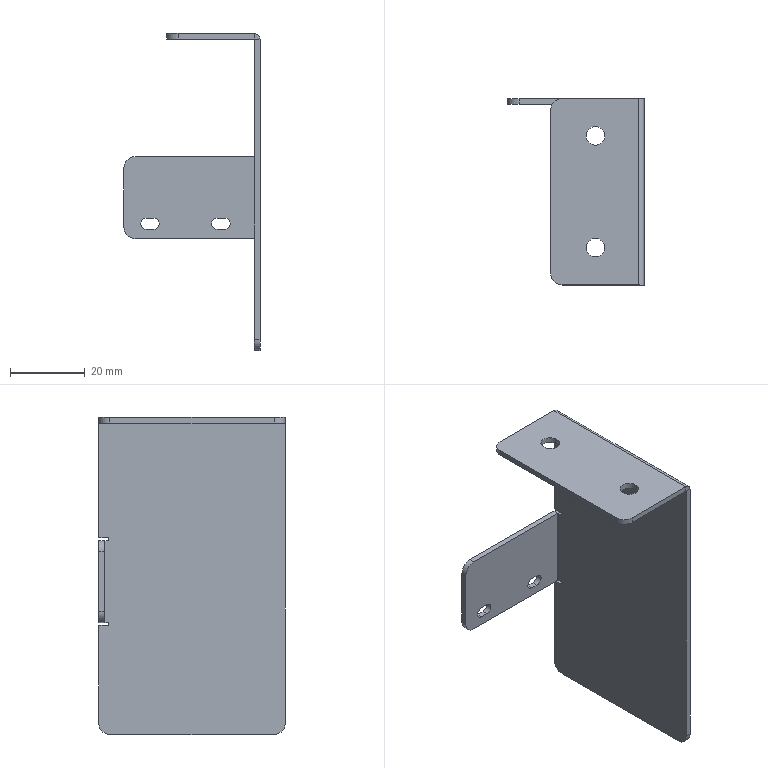Part | SolidWorks | features EdgeFlange 2, HoleWzd 2, Fillet 1, FlatPattern 1, SMBaseFlange 1, SheetMetal 1 | 1 solid | 48 faces | box 36.5 x 50 x 85 mm | volume 9132 mm3 | plane 28 | cylinder 20 | commonest cylinder face diameters 6 x6 3 x4 5 x4 0.2 x2 0.75 x2 3.2 x2
STEP:
#1=CARTESIAN_POINT('',(-15.5,15.,26.5));
#2=VERTEX_POINT('',#1);
#3=CARTESIAN_POINT('',(-10.5,15.,26.5));
#4=VERTEX_POINT('',#3);
#5=CARTESIAN_POINT('',(-13.,15.,26.5));
#6=DIRECTION('',(0.,0.,1.));
#7=DIRECTION('',(1.,0.,0.));
#8=AXIS2_PLACEMENT_3D('',#5,#6,#7);
#9=CIRCLE('',#8,2.5);
#10=EDGE_CURVE('',#2,#4,#9,.T.);
#11=ORIENTED_EDGE('',*,*,#10,.F.);
#12=CARTESIAN_POINT('',(-15.5,15.,28.));
#13=VERTEX_POINT('',#12);
#14=CARTESIAN_POINT('',(-15.5,15.,28.));
#15=DIRECTION('',(0.,0.,1.));
#16=VECTOR('',#15,1000.);
#17=LINE('',#14,#16);
#18=EDGE_CURVE('',#2,#13,#17,.T.);
#19=ORIENTED_EDGE('',*,*,#18,.T.);
#20=CARTESIAN_POINT('',(-10.5,15.,28.));
#21=VERTEX_POINT('',#20);
#22=CARTESIAN_POINT('',(-13.,15.,28.));
#23=DIRECTION('',(0.,0.,1.));
#24=DIRECTION('',(1.,0.,0.));
#25=AXIS2_PLACEMENT_3D('',#22,#23,#24);
#26=CIRCLE('',#25,2.5);
#27=EDGE_CURVE('',#13,#21,#26,.T.);
#28=ORIENTED_EDGE('',*,*,#27,.T.);
#29=CARTESIAN_POINT('',(-10.5,15.,28.));
#30=DIRECTION('',(0.,0.,1.));
#31=VECTOR('',#30,1000.);
#32=LINE('',#29,#31);
#33=EDGE_CURVE('',#4,#21,#32,.T.);
#34=ORIENTED_EDGE('',*,*,#33,.F.);
#35=EDGE_LOOP('',(#11,#19,#28,#34));
#36=FACE_OUTER_BOUND('',#35,.T.);
#37=CARTESIAN_POINT('',(-13.,15.,28.));
#38=DIRECTION('',(0.,0.,1.));
#39=DIRECTION('',(1.,0.,0.));
#40=AXIS2_PLACEMENT_3D('',#37,#38,#39);
#41=CYLINDRICAL_SURFACE('',#40,2.5);
#42=ADVANCED_FACE('',(#36),#41,.F.);
#43=CARTESIAN_POINT('',(-15.5,-15.,26.5));
#44=VERTEX_POINT('',#43);
#45=CARTESIAN_POINT('',(-10.5,-15.,26.5));
#46=VERTEX_POINT('',#45);
#47=CARTESIAN_POINT('',(-13.,-15.,26.5));
#48=DIRECTION('',(0.,0.,1.));
#49=DIRECTION('',(1.,0.,0.));
#50=AXIS2_PLACEMENT_3D('',#47,#48,#49);
#51=CIRCLE('',#50,2.5);
#52=EDGE_CURVE('',#44,#46,#51,.T.);
#53=ORIENTED_EDGE('',*,*,#52,.F.);
#54=CARTESIAN_POINT('',(-15.5,-15.,28.));
#55=VERTEX_POINT('',#54);
#56=CARTESIAN_POINT('',(-15.5,-15.,28.));
#57=DIRECTION('',(0.,0.,1.));
#58=VECTOR('',#57,1000.);
#59=LINE('',#56,#58);
#60=EDGE_CURVE('',#44,#55,#59,.T.);
#61=ORIENTED_EDGE('',*,*,#60,.T.);
#62=CARTESIAN_POINT('',(-10.5,-15.,28.));
#63=VERTEX_POINT('',#62);
#64=CARTESIAN_POINT('',(-13.,-15.,28.));
#65=DIRECTION('',(0.,0.,1.));
#66=DIRECTION('',(1.,0.,0.));
#67=AXIS2_PLACEMENT_3D('',#64,#65,#66);
#68=CIRCLE('',#67,2.5);
#69=EDGE_CURVE('',#55,#63,#68,.T.);
#70=ORIENTED_EDGE('',*,*,#69,.T.);
#71=CARTESIAN_POINT('',(-10.5,-15.,28.));
#72=DIRECTION('',(0.,0.,1.));
#73=VECTOR('',#72,1000.);
#74=LINE('',#71,#73);
#75=EDGE_CURVE('',#46,#63,#74,.T.);
#76=ORIENTED_EDGE('',*,*,#75,.F.);
#77=EDGE_LOOP('',(#53,#61,#70,#76));
#78=FACE_OUTER_BOUND('',#77,.T.);
#79=CARTESIAN_POINT('',(-13.,-15.,28.));
#80=DIRECTION('',(0.,0.,1.));
#81=DIRECTION('',(1.,0.,0.));
#82=AXIS2_PLACEMENT_3D('',#79,#80,#81);
#83=CYLINDRICAL_SURFACE('',#82,2.5);
#84=ADVANCED_FACE('',(#78),#83,.F.);
#85=CARTESIAN_POINT('',(0.,25.,-54.));
#86=VERTEX_POINT('',#85);
#87=CARTESIAN_POINT('',(0.,25.,-27.75));
#88=VERTEX_POINT('',#87);
#89=CARTESIAN_POINT('',(0.,25.,-57.));
#90=DIRECTION('',(0.,0.,1.));
#91=VECTOR('',#90,1000.);
#92=LINE('',#89,#91);
#93=EDGE_CURVE('',#86,#88,#92,.T.);
#94=ORIENTED_EDGE('',*,*,#93,.F.);
#95=CARTESIAN_POINT('',(-1.5,25.,-54.));
#96=VERTEX_POINT('',#95);
#97=CARTESIAN_POINT('',(-1.5,25.,-54.));
#98=DIRECTION('',(-1.,0.,0.));
#99=VECTOR('',#98,1000.);
#100=LINE('',#97,#99);
#101=EDGE_CURVE('',#86,#96,#100,.T.);
#102=ORIENTED_EDGE('',*,*,#101,.T.);
#103=CARTESIAN_POINT('',(-1.5,25.,-27.75));
#104=VERTEX_POINT('',#103);
#105=CARTESIAN_POINT('',(-1.5,25.,-57.));
#106=DIRECTION('',(0.,0.,1.));
#107=VECTOR('',#106,1000.);
#108=LINE('',#105,#107);
#109=EDGE_CURVE('',#96,#104,#108,.T.);
#110=ORIENTED_EDGE('',*,*,#109,.T.);
#111=CARTESIAN_POINT('',(-1.5,25.,-27.75));
#112=DIRECTION('',(1.,0.,0.));
#113=VECTOR('',#112,1000.);
#114=LINE('',#111,#113);
#115=EDGE_CURVE('',#104,#88,#114,.T.);
#116=ORIENTED_EDGE('',*,*,#115,.T.);
#117=EDGE_LOOP('',(#94,#102,#110,#116));
#118=FACE_OUTER_BOUND('',#117,.T.);
#119=CARTESIAN_POINT('',(-1.5,25.,-57.));
#120=DIRECTION('',(0.,1.,0.));
#121=DIRECTION('',(0.,0.,1.));
#122=AXIS2_PLACEMENT_3D('',#119,#120,#121);
#123=PLANE('',#122);
#124=ADVANCED_FACE('',(#118),#123,.T.);
#125=CARTESIAN_POINT('',(0.,25.,-4.25));
#126=VERTEX_POINT('',#125);
#127=CARTESIAN_POINT('',(0.,25.,26.4));
#128=VERTEX_POINT('',#127);
#129=CARTESIAN_POINT('',(0.,25.,-57.));
#130=DIRECTION('',(0.,0.,1.));
#131=VECTOR('',#130,1000.);
#132=LINE('',#129,#131);
#133=EDGE_CURVE('',#126,#128,#132,.T.);
#134=ORIENTED_EDGE('',*,*,#133,.F.);
#135=CARTESIAN_POINT('',(-1.5,25.,-4.25));
#136=VERTEX_POINT('',#135);
#137=CARTESIAN_POINT('',(-1.5,25.,-4.25));
#138=DIRECTION('',(1.,0.,0.));
#139=VECTOR('',#138,1000.);
#140=LINE('',#137,#139);
#141=EDGE_CURVE('',#136,#126,#140,.T.);
#142=ORIENTED_EDGE('',*,*,#141,.F.);
#143=CARTESIAN_POINT('',(-1.5,25.,26.4));
#144=VERTEX_POINT('',#143);
#145=CARTESIAN_POINT('',(-1.5,25.,-57.));
#146=DIRECTION('',(0.,0.,1.));
#147=VECTOR('',#146,1000.);
#148=LINE('',#145,#147);
#149=EDGE_CURVE('',#136,#144,#148,.T.);
#150=ORIENTED_EDGE('',*,*,#149,.T.);
#151=CARTESIAN_POINT('',(-1.5,25.,26.4));
#152=DIRECTION('',(1.,0.,0.));
#153=VECTOR('',#152,1000.);
#154=LINE('',#151,#153);
#155=EDGE_CURVE('',#144,#128,#154,.T.);
#156=ORIENTED_EDGE('',*,*,#155,.T.);
#157=EDGE_LOOP('',(#134,#142,#150,#156));
#158=FACE_OUTER_BOUND('',#157,.T.);
#159=CARTESIAN_POINT('',(-1.5,25.,-57.));
#160=DIRECTION('',(0.,1.,0.));
#161=DIRECTION('',(0.,0.,1.));
#162=AXIS2_PLACEMENT_3D('',#159,#160,#161);
#163=PLANE('',#162);
#164=ADVANCED_FACE('',(#158),#163,.T.);
#165=CARTESIAN_POINT('',(-1.5,-22.,-57.));
#166=VERTEX_POINT('',#165);
#167=CARTESIAN_POINT('',(-1.5,22.,-57.));
#168=VERTEX_POINT('',#167);
#169=CARTESIAN_POINT('',(-1.5,-25.,-57.));
#170=DIRECTION('',(0.,1.,0.));
#171=VECTOR('',#170,1000.);
#172=LINE('',#169,#171);
#173=EDGE_CURVE('',#166,#168,#172,.T.);
#174=ORIENTED_EDGE('',*,*,#173,.F.);
#175=CARTESIAN_POINT('',(-1.5,-25.,-54.));
#176=VERTEX_POINT('',#175);
#177=CARTESIAN_POINT('',(-1.5,-22.,-54.));
#178=DIRECTION('',(-1.,0.,0.));
#179=DIRECTION('',(0.,0.,-1.));
#180=AXIS2_PLACEMENT_3D('',#177,#178,#179);
#181=CIRCLE('',#180,3.);
#182=EDGE_CURVE('',#166,#176,#181,.T.);
#183=ORIENTED_EDGE('',*,*,#182,.T.);
#184=CARTESIAN_POINT('',(-1.5,-25.,26.4));
#185=VERTEX_POINT('',#184);
#186=CARTESIAN_POINT('',(-1.5,-25.,-57.));
#187=DIRECTION('',(0.,0.,-1.));
#188=VECTOR('',#187,1000.);
#189=LINE('',#186,#188);
#190=EDGE_CURVE('',#185,#176,#189,.T.);
#191=ORIENTED_EDGE('',*,*,#190,.F.);
#192=CARTESIAN_POINT('',(-1.5,25.,26.4));
#193=DIRECTION('',(0.,-1.,0.));
#194=VECTOR('',#193,1000.);
#195=LINE('',#192,#194);
#196=EDGE_CURVE('',#144,#185,#195,.T.);
#197=ORIENTED_EDGE('',*,*,#196,.F.);
#198=ORIENTED_EDGE('',*,*,#149,.F.);
#199=CARTESIAN_POINT('',(-1.5,22.65,-4.25));
#200=VERTEX_POINT('',#199);
#201=CARTESIAN_POINT('',(-1.5,22.65,-4.25));
#202=DIRECTION('',(0.,1.,0.));
#203=VECTOR('',#202,1000.);
#204=LINE('',#201,#203);
#205=EDGE_CURVE('',#200,#136,#204,.T.);
#206=ORIENTED_EDGE('',*,*,#205,.F.);
#207=CARTESIAN_POINT('',(-1.5,22.65,-5.));
#208=VERTEX_POINT('',#207);
#209=CARTESIAN_POINT('',(-1.5,22.65,-4.625));
#210=DIRECTION('',(-1.,0.,0.));
#211=DIRECTION('',(0.,0.,1.));
#212=AXIS2_PLACEMENT_3D('',#209,#210,#211);
#213=CIRCLE('',#212,0.375);
#214=EDGE_CURVE('',#208,#200,#213,.T.);
#215=ORIENTED_EDGE('',*,*,#214,.F.);
#216=CARTESIAN_POINT('',(-1.5,23.4,-5.));
#217=VERTEX_POINT('',#216);
#218=CARTESIAN_POINT('',(-1.5,23.4,-5.));
#219=DIRECTION('',(0.,-1.,0.));
#220=VECTOR('',#219,1000.);
#221=LINE('',#218,#220);
#222=EDGE_CURVE('',#217,#208,#221,.T.);
#223=ORIENTED_EDGE('',*,*,#222,.F.);
#224=CARTESIAN_POINT('',(-1.5,23.4,-27.));
#225=VERTEX_POINT('',#224);
#226=CARTESIAN_POINT('',(-1.5,23.4,-27.));
#227=DIRECTION('',(0.,0.,1.));
#228=VECTOR('',#227,1000.);
#229=LINE('',#226,#228);
#230=EDGE_CURVE('',#225,#217,#229,.T.);
#231=ORIENTED_EDGE('',*,*,#230,.F.);
#232=CARTESIAN_POINT('',(-1.5,22.65,-27.));
#233=VERTEX_POINT('',#232);
#234=CARTESIAN_POINT('',(-1.5,22.65,-27.));
#235=DIRECTION('',(0.,1.,0.));
#236=VECTOR('',#235,1000.);
#237=LINE('',#234,#236);
#238=EDGE_CURVE('',#233,#225,#237,.T.);
#239=ORIENTED_EDGE('',*,*,#238,.F.);
#240=CARTESIAN_POINT('',(-1.5,22.65,-27.75));
#241=VERTEX_POINT('',#240);
#242=CARTESIAN_POINT('',(-1.5,22.65,-27.375));
#243=DIRECTION('',(-1.,0.,0.));
#244=DIRECTION('',(0.,0.,1.));
#245=AXIS2_PLACEMENT_3D('',#242,#243,#244);
#246=CIRCLE('',#245,0.375);
#247=EDGE_CURVE('',#241,#233,#246,.T.);
#248=ORIENTED_EDGE('',*,*,#247,.F.);
#249=CARTESIAN_POINT('',(-1.5,25.,-27.75));
#250=DIRECTION('',(0.,-1.,0.));
#251=VECTOR('',#250,1000.);
#252=LINE('',#249,#251);
#253=EDGE_CURVE('',#104,#241,#252,.T.);
#254=ORIENTED_EDGE('',*,*,#253,.F.);
#255=ORIENTED_EDGE('',*,*,#109,.F.);
#256=CARTESIAN_POINT('',(-1.5,22.,-54.));
#257=DIRECTION('',(-1.,0.,0.));
#258=DIRECTION('',(0.,0.,-1.));
#259=AXIS2_PLACEMENT_3D('',#256,#257,#258);
#260=CIRCLE('',#259,3.);
#261=EDGE_CURVE('',#96,#168,#260,.T.);
#262=ORIENTED_EDGE('',*,*,#261,.T.);
#263=EDGE_LOOP('',(#174,#183,#191,#197,#198,#206,#215,#223,#231,#239,#248,#254,#255,#262));
#264=FACE_OUTER_BOUND('',#263,.T.);
#265=CARTESIAN_POINT('',(-1.5,0.,0.));
#266=DIRECTION('',(1.,0.,0.));
#267=DIRECTION('',(0.,0.,-1.));
#268=AXIS2_PLACEMENT_3D('',#265,#266,#267);
#269=PLANE('',#268);
#270=ADVANCED_FACE('',(#264),#269,.F.);
#271=CARTESIAN_POINT('',(0.,-25.,26.4));
#272=VERTEX_POINT('',#271);
#273=CARTESIAN_POINT('',(0.,-25.,-54.));
#274=VERTEX_POINT('',#273);
#275=CARTESIAN_POINT('',(0.,-25.,-57.));
#276=DIRECTION('',(0.,0.,-1.));
#277=VECTOR('',#276,1000.);
#278=LINE('',#275,#277);
#279=EDGE_CURVE('',#272,#274,#278,.T.);
#280=ORIENTED_EDGE('',*,*,#279,.T.);
#281=CARTESIAN_POINT('',(0.,-22.,-57.));
#282=VERTEX_POINT('',#281);
#283=CARTESIAN_POINT('',(0.,-22.,-54.));
#284=DIRECTION('',(1.,0.,0.));
#285=DIRECTION('',(0.,0.,-1.));
#286=AXIS2_PLACEMENT_3D('',#283,#284,#285);
#287=CIRCLE('',#286,3.);
#288=EDGE_CURVE('',#274,#282,#287,.T.);
#289=ORIENTED_EDGE('',*,*,#288,.T.);
#290=CARTESIAN_POINT('',(0.,22.,-57.));
#291=VERTEX_POINT('',#290);
#292=CARTESIAN_POINT('',(0.,-25.,-57.));
#293=DIRECTION('',(0.,1.,0.));
#294=VECTOR('',#293,1000.);
#295=LINE('',#292,#294);
#296=EDGE_CURVE('',#282,#291,#295,.T.);
#297=ORIENTED_EDGE('',*,*,#296,.T.);
#298=CARTESIAN_POINT('',(0.,22.,-54.));
#299=DIRECTION('',(1.,0.,0.));
#300=DIRECTION('',(0.,0.,-1.));
#301=AXIS2_PLACEMENT_3D('',#298,#299,#300);
#302=CIRCLE('',#301,3.);
#303=EDGE_CURVE('',#291,#86,#302,.T.);
#304=ORIENTED_EDGE('',*,*,#303,.T.);
#305=ORIENTED_EDGE('',*,*,#93,.T.);
#306=CARTESIAN_POINT('',(0.,22.65,-27.75));
#307=VERTEX_POINT('',#306);
#308=CARTESIAN_POINT('',(0.,0.,-27.75));
#309=DIRECTION('',(0.,-1.,0.));
#310=VECTOR('',#309,1000.);
#311=LINE('',#308,#310);
#312=EDGE_CURVE('',#88,#307,#311,.T.);
#313=ORIENTED_EDGE('',*,*,#312,.T.);
#314=CARTESIAN_POINT('',(0.,22.65,-27.));
#315=VERTEX_POINT('',#314);
#316=CARTESIAN_POINT('',(0.,22.65,-27.375));
#317=DIRECTION('',(-1.,0.,0.));
#318=DIRECTION('',(0.,0.,-1.));
#319=AXIS2_PLACEMENT_3D('',#316,#317,#318);
#320=CIRCLE('',#319,0.375);
#321=EDGE_CURVE('',#307,#315,#320,.T.);
#322=ORIENTED_EDGE('',*,*,#321,.T.);
#323=CARTESIAN_POINT('',(0.,23.4,-27.));
#324=VERTEX_POINT('',#323);
#325=CARTESIAN_POINT('',(0.,0.,-27.));
#326=DIRECTION('',(0.,1.,0.));
#327=VECTOR('',#326,1000.);
#328=LINE('',#325,#327);
#329=EDGE_CURVE('',#315,#324,#328,.T.);
#330=ORIENTED_EDGE('',*,*,#329,.T.);
#331=CARTESIAN_POINT('',(0.,23.4,-5.));
#332=VERTEX_POINT('',#331);
#333=CARTESIAN_POINT('',(0.,23.4,-27.));
#334=DIRECTION('',(0.,0.,1.));
#335=VECTOR('',#334,1000.);
#336=LINE('',#333,#335);
#337=EDGE_CURVE('',#324,#332,#336,.T.);
#338=ORIENTED_EDGE('',*,*,#337,.T.);
#339=CARTESIAN_POINT('',(0.,22.65,-5.));
#340=VERTEX_POINT('',#339);
#341=CARTESIAN_POINT('',(0.,0.,-5.));
#342=DIRECTION('',(0.,-1.,0.));
#343=VECTOR('',#342,1000.);
#344=LINE('',#341,#343);
#345=EDGE_CURVE('',#332,#340,#344,.T.);
#346=ORIENTED_EDGE('',*,*,#345,.T.);
#347=CARTESIAN_POINT('',(0.,22.65,-4.25));
#348=VERTEX_POINT('',#347);
#349=CARTESIAN_POINT('',(0.,22.65,-4.625));
#350=DIRECTION('',(-1.,0.,0.));
#351=DIRECTION('',(0.,0.,-1.));
#352=AXIS2_PLACEMENT_3D('',#349,#350,#351);
#353=CIRCLE('',#352,0.375);
#354=EDGE_CURVE('',#340,#348,#353,.T.);
#355=ORIENTED_EDGE('',*,*,#354,.T.);
#356=CARTESIAN_POINT('',(0.,0.,-4.25));
#357=DIRECTION('',(0.,1.,0.));
#358=VECTOR('',#357,1000.);
#359=LINE('',#356,#358);
#360=EDGE_CURVE('',#348,#126,#359,.T.);
#361=ORIENTED_EDGE('',*,*,#360,.T.);
#362=ORIENTED_EDGE('',*,*,#133,.T.);
#363=CARTESIAN_POINT('',(0.,25.,26.4));
#364=DIRECTION('',(0.,-1.,0.));
#365=VECTOR('',#364,1000.);
#366=LINE('',#363,#365);
#367=EDGE_CURVE('',#128,#272,#366,.T.);
#368=ORIENTED_EDGE('',*,*,#367,.T.);
#369=EDGE_LOOP('',(#280,#289,#297,#304,#305,#313,#322,#330,#338,#346,#355,#361,#362,#368));
#370=FACE_OUTER_BOUND('',#369,.T.);
#371=CARTESIAN_POINT('',(0.,0.,0.));
#372=DIRECTION('',(1.,0.,0.));
#373=DIRECTION('',(0.,0.,-1.));
#374=AXIS2_PLACEMENT_3D('',#371,#372,#373);
#375=PLANE('',#374);
#376=ADVANCED_FACE('',(#370),#375,.T.);
#377=ORIENTED_EDGE('',*,*,#296,.F.);
#378=CARTESIAN_POINT('',(-1.5,-22.,-57.));
#379=DIRECTION('',(-1.,0.,0.));
#380=VECTOR('',#379,1000.);
#381=LINE('',#378,#380);
#382=EDGE_CURVE('',#282,#166,#381,.T.);
#383=ORIENTED_EDGE('',*,*,#382,.T.);
#384=ORIENTED_EDGE('',*,*,#173,.T.);
#385=CARTESIAN_POINT('',(-1.5,22.,-57.));
#386=DIRECTION('',(1.,0.,0.));
#387=VECTOR('',#386,1000.);
#388=LINE('',#385,#387);
#389=EDGE_CURVE('',#168,#291,#388,.T.);
#390=ORIENTED_EDGE('',*,*,#389,.T.);
#391=EDGE_LOOP('',(#377,#383,#384,#390));
#392=FACE_OUTER_BOUND('',#391,.T.);
#393=CARTESIAN_POINT('',(-1.5,-25.,-57.));
#394=DIRECTION('',(0.,0.,-1.));
#395=DIRECTION('',(-1.,0.,0.));
#396=AXIS2_PLACEMENT_3D('',#393,#394,#395);
#397=PLANE('',#396);
#398=ADVANCED_FACE('',(#392),#397,.T.);
#399=ORIENTED_EDGE('',*,*,#190,.T.);
#400=CARTESIAN_POINT('',(-1.5,-25.,-54.));
#401=DIRECTION('',(1.,0.,0.));
#402=VECTOR('',#401,1000.);
#403=LINE('',#400,#402);
#404=EDGE_CURVE('',#176,#274,#403,.T.);
#405=ORIENTED_EDGE('',*,*,#404,.T.);
#406=ORIENTED_EDGE('',*,*,#279,.F.);
#407=CARTESIAN_POINT('',(-1.5,-25.,26.4));
#408=DIRECTION('',(1.,0.,0.));
#409=VECTOR('',#408,1000.);
#410=LINE('',#407,#409);
#411=EDGE_CURVE('',#185,#272,#410,.T.);
#412=ORIENTED_EDGE('',*,*,#411,.F.);
#413=EDGE_LOOP('',(#399,#405,#406,#412));
#414=FACE_OUTER_BOUND('',#413,.T.);
#415=CARTESIAN_POINT('',(-1.5,-25.,-57.));
#416=DIRECTION('',(0.,-1.,0.));
#417=DIRECTION('',(0.,0.,-1.));
#418=AXIS2_PLACEMENT_3D('',#415,#416,#417);
#419=PLANE('',#418);
#420=ADVANCED_FACE('',(#414),#419,.T.);
#421=CARTESIAN_POINT('',(-1.6,-25.,26.5));
#422=VERTEX_POINT('',#421);
#423=CARTESIAN_POINT('',(-1.6,-25.,28.));
#424=VERTEX_POINT('',#423);
#425=CARTESIAN_POINT('',(-1.6,-25.,28.));
#426=DIRECTION('',(0.,0.,1.));
#427=VECTOR('',#426,1000.);
#428=LINE('',#425,#427);
#429=EDGE_CURVE('',#422,#424,#428,.T.);
#430=ORIENTED_EDGE('',*,*,#429,.F.);
#431=CARTESIAN_POINT('',(-1.6,-25.,26.4));
#432=DIRECTION('',(0.,-1.,0.));
#433=DIRECTION('',(0.,0.,1.));
#434=AXIS2_PLACEMENT_3D('',#431,#432,#433);
#435=CIRCLE('',#434,0.1);
#436=EDGE_CURVE('',#185,#422,#435,.T.);
#437=ORIENTED_EDGE('',*,*,#436,.F.);
#438=ORIENTED_EDGE('',*,*,#411,.T.);
#439=CARTESIAN_POINT('',(-1.6,-25.,26.4));
#440=DIRECTION('',(0.,-1.,0.));
#441=DIRECTION('',(0.,0.,1.));
#442=AXIS2_PLACEMENT_3D('',#439,#440,#441);
#443=CIRCLE('',#442,1.6);
#444=EDGE_CURVE('',#272,#424,#443,.T.);
#445=ORIENTED_EDGE('',*,*,#444,.T.);
#446=EDGE_LOOP('',(#430,#437,#438,#445));
#447=FACE_OUTER_BOUND('',#446,.T.);
#448=CARTESIAN_POINT('',(-1.6,-25.,26.4));
#449=DIRECTION('',(0.,-1.,0.));
#450=DIRECTION('',(0.,0.,-1.));
#451=AXIS2_PLACEMENT_3D('',#448,#449,#450);
#452=PLANE('',#451);
#453=ADVANCED_FACE('',(#447),#452,.T.);
#454=CARTESIAN_POINT('',(-1.6,25.,26.5));
#455=VERTEX_POINT('',#454);
#456=CARTESIAN_POINT('',(-1.6,25.,26.4));
#457=DIRECTION('',(0.,1.,0.));
#458=DIRECTION('',(0.,0.,1.));
#459=AXIS2_PLACEMENT_3D('',#456,#457,#458);
#460=CIRCLE('',#459,0.1);
#461=EDGE_CURVE('',#455,#144,#460,.T.);
#462=ORIENTED_EDGE('',*,*,#461,.F.);
#463=CARTESIAN_POINT('',(-1.6,25.,28.));
#464=VERTEX_POINT('',#463);
#465=CARTESIAN_POINT('',(-1.6,25.,26.5));
#466=DIRECTION('',(0.,0.,1.));
#467=VECTOR('',#466,1000.);
#468=LINE('',#465,#467);
#469=EDGE_CURVE('',#455,#464,#468,.T.);
#470=ORIENTED_EDGE('',*,*,#469,.T.);
#471=CARTESIAN_POINT('',(-1.6,25.,26.4));
#472=DIRECTION('',(0.,1.,0.));
#473=DIRECTION('',(0.,0.,1.));
#474=AXIS2_PLACEMENT_3D('',#471,#472,#473);
#475=CIRCLE('',#474,1.6);
#476=EDGE_CURVE('',#464,#128,#475,.T.);
#477=ORIENTED_EDGE('',*,*,#476,.T.);
#478=ORIENTED_EDGE('',*,*,#155,.F.);
#479=EDGE_LOOP('',(#462,#470,#477,#478));
#480=FACE_OUTER_BOUND('',#479,.T.);
#481=CARTESIAN_POINT('',(-1.6,25.,26.4));
#482=DIRECTION('',(0.,-1.,0.));
#483=DIRECTION('',(0.,0.,-1.));
#484=AXIS2_PLACEMENT_3D('',#481,#482,#483);
#485=PLANE('',#484);
#486=ADVANCED_FACE('',(#480),#485,.F.);
#487=ORIENTED_EDGE('',*,*,#367,.F.);
#488=ORIENTED_EDGE('',*,*,#476,.F.);
#489=CARTESIAN_POINT('',(-1.6,0.,28.));
#490=DIRECTION('',(0.,1.,0.));
#491=VECTOR('',#490,1000.);
#492=LINE('',#489,#491);
#493=EDGE_CURVE('',#424,#464,#492,.T.);
#494=ORIENTED_EDGE('',*,*,#493,.F.);
#495=ORIENTED_EDGE('',*,*,#444,.F.);
#496=EDGE_LOOP('',(#487,#488,#494,#495));
#497=FACE_OUTER_BOUND('',#496,.T.);
#498=CARTESIAN_POINT('',(-1.6,25.,26.4));
#499=DIRECTION('',(0.,1.,0.));
#500=DIRECTION('',(0.,0.,1.));
#501=AXIS2_PLACEMENT_3D('',#498,#499,#500);
#502=CYLINDRICAL_SURFACE('',#501,1.6);
#503=ADVANCED_FACE('',(#497),#502,.T.);
#504=ORIENTED_EDGE('',*,*,#196,.T.);
#505=ORIENTED_EDGE('',*,*,#436,.T.);
#506=CARTESIAN_POINT('',(-1.6,-25.,26.5));
#507=DIRECTION('',(0.,1.,0.));
#508=VECTOR('',#507,1000.);
#509=LINE('',#506,#508);
#510=EDGE_CURVE('',#422,#455,#509,.T.);
#511=ORIENTED_EDGE('',*,*,#510,.T.);
#512=ORIENTED_EDGE('',*,*,#461,.T.);
#513=EDGE_LOOP('',(#504,#505,#511,#512));
#514=FACE_OUTER_BOUND('',#513,.T.);
#515=CARTESIAN_POINT('',(-1.6,25.,26.4));
#516=DIRECTION('',(0.,1.,0.));
#517=DIRECTION('',(0.,0.,1.));
#518=AXIS2_PLACEMENT_3D('',#515,#516,#517);
#519=CYLINDRICAL_SURFACE('',#518,0.1);
#520=ADVANCED_FACE('',(#514),#519,.F.);
#521=CARTESIAN_POINT('',(-22.,25.,26.5));
#522=VERTEX_POINT('',#521);
#523=CARTESIAN_POINT('',(0.,25.,26.5));
#524=DIRECTION('',(1.,0.,0.));
#525=VECTOR('',#524,1000.);
#526=LINE('',#523,#525);
#527=EDGE_CURVE('',#522,#455,#526,.T.);
#528=ORIENTED_EDGE('',*,*,#527,.F.);
#529=CARTESIAN_POINT('',(-22.,25.,28.));
#530=VERTEX_POINT('',#529);
#531=CARTESIAN_POINT('',(-22.,25.,28.));
#532=DIRECTION('',(0.,0.,1.));
#533=VECTOR('',#532,1000.);
#534=LINE('',#531,#533);
#535=EDGE_CURVE('',#522,#530,#534,.T.);
#536=ORIENTED_EDGE('',*,*,#535,.T.);
#537=CARTESIAN_POINT('',(-1.5,25.,28.));
#538=DIRECTION('',(1.,0.,0.));
#539=VECTOR('',#538,1000.);
#540=LINE('',#537,#539);
#541=EDGE_CURVE('',#530,#464,#540,.T.);
#542=ORIENTED_EDGE('',*,*,#541,.T.);
#543=ORIENTED_EDGE('',*,*,#469,.F.);
#544=EDGE_LOOP('',(#528,#536,#542,#543));
#545=FACE_OUTER_BOUND('',#544,.T.);
#546=CARTESIAN_POINT('',(-1.5,25.,28.));
#547=DIRECTION('',(0.,1.,0.));
#548=DIRECTION('',(-1.,0.,0.));
#549=AXIS2_PLACEMENT_3D('',#546,#547,#548);
#550=PLANE('',#549);
#551=ADVANCED_FACE('',(#545),#550,.T.);
#552=CARTESIAN_POINT('',(-22.,-25.,28.));
#553=VERTEX_POINT('',#552);
#554=CARTESIAN_POINT('',(-25.,-25.,28.));
#555=DIRECTION('',(-1.,0.,0.));
#556=VECTOR('',#555,1000.);
#557=LINE('',#554,#556);
#558=EDGE_CURVE('',#424,#553,#557,.T.);
#559=ORIENTED_EDGE('',*,*,#558,.T.);
#560=CARTESIAN_POINT('',(-22.,-25.,26.5));
#561=VERTEX_POINT('',#560);
#562=CARTESIAN_POINT('',(-22.,-25.,28.));
#563=DIRECTION('',(0.,0.,-1.));
#564=VECTOR('',#563,1000.);
#565=LINE('',#562,#564);
#566=EDGE_CURVE('',#553,#561,#565,.T.);
#567=ORIENTED_EDGE('',*,*,#566,.T.);
#568=CARTESIAN_POINT('',(0.,-25.,26.5));
#569=DIRECTION('',(-1.,0.,0.));
#570=VECTOR('',#569,1000.);
#571=LINE('',#568,#570);
#572=EDGE_CURVE('',#422,#561,#571,.T.);
#573=ORIENTED_EDGE('',*,*,#572,.F.);
#574=ORIENTED_EDGE('',*,*,#429,.T.);
#575=EDGE_LOOP('',(#559,#567,#573,#574));
#576=FACE_OUTER_BOUND('',#575,.T.);
#577=CARTESIAN_POINT('',(-25.,-25.,28.));
#578=DIRECTION('',(0.,-1.,0.));
#579=DIRECTION('',(1.,0.,0.));
#580=AXIS2_PLACEMENT_3D('',#577,#578,#579);
#581=PLANE('',#580);
#582=ADVANCED_FACE('',(#576),#581,.T.);
#583=CARTESIAN_POINT('',(-13.,15.,28.));
#584=DIRECTION('',(0.,0.,1.));
#585=DIRECTION('',(1.,0.,0.));
#586=AXIS2_PLACEMENT_3D('',#583,#584,#585);
#587=CIRCLE('',#586,2.5);
#588=EDGE_CURVE('',#21,#13,#587,.T.);
#589=ORIENTED_EDGE('',*,*,#588,.F.);
#590=ORIENTED_EDGE('',*,*,#27,.F.);
#591=EDGE_LOOP('',(#589,#590));
#592=FACE_BOUND('',#591,.T.);
#593=CARTESIAN_POINT('',(-13.,-15.,28.));
#594=DIRECTION('',(0.,0.,1.));
#595=DIRECTION('',(1.,0.,0.));
#596=AXIS2_PLACEMENT_3D('',#593,#594,#595);
#597=CIRCLE('',#596,2.5);
#598=EDGE_CURVE('',#63,#55,#597,.T.);
#599=ORIENTED_EDGE('',*,*,#598,.F.);
#600=ORIENTED_EDGE('',*,*,#69,.F.);
#601=EDGE_LOOP('',(#599,#600));
#602=FACE_BOUND('',#601,.T.);
#603=CARTESIAN_POINT('',(-25.,-22.,28.));
#604=VERTEX_POINT('',#603);
#605=CARTESIAN_POINT('',(-25.,22.,28.));
#606=VERTEX_POINT('',#605);
#607=CARTESIAN_POINT('',(-25.,25.,28.));
#608=DIRECTION('',(0.,1.,0.));
#609=VECTOR('',#608,1000.);
#610=LINE('',#607,#609);
#611=EDGE_CURVE('',#604,#606,#610,.T.);
#612=ORIENTED_EDGE('',*,*,#611,.F.);
#613=CARTESIAN_POINT('',(-22.,-22.,28.));
#614=DIRECTION('',(0.,0.,1.));
#615=DIRECTION('',(1.,0.,0.));
#616=AXIS2_PLACEMENT_3D('',#613,#614,#615);
#617=CIRCLE('',#616,3.);
#618=EDGE_CURVE('',#604,#553,#617,.T.);
#619=ORIENTED_EDGE('',*,*,#618,.T.);
#620=ORIENTED_EDGE('',*,*,#558,.F.);
#621=ORIENTED_EDGE('',*,*,#493,.T.);
#622=ORIENTED_EDGE('',*,*,#541,.F.);
#623=CARTESIAN_POINT('',(-22.,22.,28.));
#624=DIRECTION('',(0.,0.,1.));
#625=DIRECTION('',(1.,0.,0.));
#626=AXIS2_PLACEMENT_3D('',#623,#624,#625);
#627=CIRCLE('',#626,3.);
#628=EDGE_CURVE('',#530,#606,#627,.T.);
#629=ORIENTED_EDGE('',*,*,#628,.T.);
#630=EDGE_LOOP('',(#612,#619,#620,#621,#622,#629));
#631=FACE_OUTER_BOUND('',#630,.T.);
#632=CARTESIAN_POINT('',(0.,0.,28.));
#633=DIRECTION('',(0.,0.,1.));
#634=DIRECTION('',(1.,0.,0.));
#635=AXIS2_PLACEMENT_3D('',#632,#633,#634);
#636=PLANE('',#635);
#637=ADVANCED_FACE('',(#592,#602,#631),#636,.T.);
#638=CARTESIAN_POINT('',(-13.,15.,26.5));
#639=DIRECTION('',(0.,0.,1.));
#640=DIRECTION('',(1.,0.,0.));
#641=AXIS2_PLACEMENT_3D('',#638,#639,#640);
#642=CIRCLE('',#641,2.5);
#643=EDGE_CURVE('',#4,#2,#642,.T.);
#644=ORIENTED_EDGE('',*,*,#643,.T.);
#645=ORIENTED_EDGE('',*,*,#10,.T.);
#646=EDGE_LOOP('',(#644,#645));
#647=FACE_BOUND('',#646,.T.);
#648=CARTESIAN_POINT('',(-13.,-15.,26.5));
#649=DIRECTION('',(0.,0.,1.));
#650=DIRECTION('',(1.,0.,0.));
#651=AXIS2_PLACEMENT_3D('',#648,#649,#650);
#652=CIRCLE('',#651,2.5);
#653=EDGE_CURVE('',#46,#44,#652,.T.);
#654=ORIENTED_EDGE('',*,*,#653,.T.);
#655=ORIENTED_EDGE('',*,*,#52,.T.);
#656=EDGE_LOOP('',(#654,#655));
#657=FACE_BOUND('',#656,.T.);
#658=ORIENTED_EDGE('',*,*,#572,.T.);
#659=CARTESIAN_POINT('',(-25.,-22.,26.5));
#660=VERTEX_POINT('',#659);
#661=CARTESIAN_POINT('',(-22.,-22.,26.5));
#662=DIRECTION('',(0.,0.,-1.));
#663=DIRECTION('',(1.,0.,0.));
#664=AXIS2_PLACEMENT_3D('',#661,#662,#663);
#665=CIRCLE('',#664,3.);
#666=EDGE_CURVE('',#561,#660,#665,.T.);
#667=ORIENTED_EDGE('',*,*,#666,.T.);
#668=CARTESIAN_POINT('',(-25.,22.,26.5));
#669=VERTEX_POINT('',#668);
#670=CARTESIAN_POINT('',(-25.,0.,26.5));
#671=DIRECTION('',(0.,1.,0.));
#672=VECTOR('',#671,1000.);
#673=LINE('',#670,#672);
#674=EDGE_CURVE('',#660,#669,#673,.T.);
#675=ORIENTED_EDGE('',*,*,#674,.T.);
#676=CARTESIAN_POINT('',(-22.,22.,26.5));
#677=DIRECTION('',(0.,0.,-1.));
#678=DIRECTION('',(1.,0.,0.));
#679=AXIS2_PLACEMENT_3D('',#676,#677,#678);
#680=CIRCLE('',#679,3.);
#681=EDGE_CURVE('',#669,#522,#680,.T.);
#682=ORIENTED_EDGE('',*,*,#681,.T.);
#683=ORIENTED_EDGE('',*,*,#527,.T.);
#684=ORIENTED_EDGE('',*,*,#510,.F.);
#685=EDGE_LOOP('',(#658,#667,#675,#682,#683,#684));
#686=FACE_OUTER_BOUND('',#685,.T.);
#687=CARTESIAN_POINT('',(0.,0.,26.5));
#688=DIRECTION('',(0.,0.,1.));
#689=DIRECTION('',(1.,0.,0.));
#690=AXIS2_PLACEMENT_3D('',#687,#688,#689);
#691=PLANE('',#690);
#692=ADVANCED_FACE('',(#647,#657,#686),#691,.F.);
#693=ORIENTED_EDGE('',*,*,#674,.F.);
#694=CARTESIAN_POINT('',(-25.,-22.,28.));
#695=DIRECTION('',(0.,0.,1.));
#696=VECTOR('',#695,1000.);
#697=LINE('',#694,#696);
#698=EDGE_CURVE('',#660,#604,#697,.T.);
#699=ORIENTED_EDGE('',*,*,#698,.T.);
#700=ORIENTED_EDGE('',*,*,#611,.T.);
#701=CARTESIAN_POINT('',(-25.,22.,28.));
#702=DIRECTION('',(0.,0.,-1.));
#703=VECTOR('',#702,1000.);
#704=LINE('',#701,#703);
#705=EDGE_CURVE('',#606,#669,#704,.T.);
#706=ORIENTED_EDGE('',*,*,#705,.T.);
#707=EDGE_LOOP('',(#693,#699,#700,#706));
#708=FACE_OUTER_BOUND('',#707,.T.);
#709=CARTESIAN_POINT('',(-25.,25.,28.));
#710=DIRECTION('',(-1.,0.,0.));
#711=DIRECTION('',(0.,0.,1.));
#712=AXIS2_PLACEMENT_3D('',#709,#710,#711);
#713=PLANE('',#712);
#714=ADVANCED_FACE('',(#708),#713,.T.);
#715=ORIENTED_EDGE('',*,*,#312,.F.);
#716=ORIENTED_EDGE('',*,*,#115,.F.);
#717=ORIENTED_EDGE('',*,*,#253,.T.);
#718=CARTESIAN_POINT('',(-1.5,22.65,-27.75));
#719=DIRECTION('',(1.,0.,0.));
#720=VECTOR('',#719,1000.);
#721=LINE('',#718,#720);
#722=EDGE_CURVE('',#241,#307,#721,.T.);
#723=ORIENTED_EDGE('',*,*,#722,.T.);
#724=EDGE_LOOP('',(#715,#716,#717,#723));
#725=FACE_OUTER_BOUND('',#724,.T.);
#726=CARTESIAN_POINT('',(-1.5,25.,-27.75));
#727=DIRECTION('',(0.,0.,1.));
#728=DIRECTION('',(1.,0.,0.));
#729=AXIS2_PLACEMENT_3D('',#726,#727,#728);
#730=PLANE('',#729);
#731=ADVANCED_FACE('',(#725),#730,.T.);
#732=ORIENTED_EDGE('',*,*,#321,.F.);
#733=ORIENTED_EDGE('',*,*,#722,.F.);
#734=ORIENTED_EDGE('',*,*,#247,.T.);
#735=CARTESIAN_POINT('',(-1.5,22.65,-27.));
#736=DIRECTION('',(1.,0.,0.));
#737=VECTOR('',#736,1000.);
#738=LINE('',#735,#737);
#739=EDGE_CURVE('',#233,#315,#738,.T.);
#740=ORIENTED_EDGE('',*,*,#739,.T.);
#741=EDGE_LOOP('',(#732,#733,#734,#740));
#742=FACE_OUTER_BOUND('',#741,.T.);
#743=CARTESIAN_POINT('',(-1.5,22.65,-27.375));
#744=DIRECTION('',(1.,0.,0.));
#745=DIRECTION('',(0.,0.,-1.));
#746=AXIS2_PLACEMENT_3D('',#743,#744,#745);
#747=CYLINDRICAL_SURFACE('',#746,0.375);
#748=ADVANCED_FACE('',(#742),#747,.F.);
#749=ORIENTED_EDGE('',*,*,#329,.F.);
#750=ORIENTED_EDGE('',*,*,#739,.F.);
#751=ORIENTED_EDGE('',*,*,#238,.T.);
#752=CARTESIAN_POINT('',(-1.5,23.4,-27.));
#753=DIRECTION('',(1.,0.,0.));
#754=VECTOR('',#753,1000.);
#755=LINE('',#752,#754);
#756=EDGE_CURVE('',#225,#324,#755,.T.);
#757=ORIENTED_EDGE('',*,*,#756,.T.);
#758=EDGE_LOOP('',(#749,#750,#751,#757));
#759=FACE_OUTER_BOUND('',#758,.T.);
#760=CARTESIAN_POINT('',(-1.5,22.65,-27.));
#761=DIRECTION('',(0.,0.,-1.));
#762=DIRECTION('',(-1.,0.,0.));
#763=AXIS2_PLACEMENT_3D('',#760,#761,#762);
#764=PLANE('',#763);
#765=ADVANCED_FACE('',(#759),#764,.T.);
#766=ORIENTED_EDGE('',*,*,#345,.F.);
#767=CARTESIAN_POINT('',(-1.5,23.4,-5.));
#768=DIRECTION('',(1.,0.,0.));
#769=VECTOR('',#768,1000.);
#770=LINE('',#767,#769);
#771=EDGE_CURVE('',#217,#332,#770,.T.);
#772=ORIENTED_EDGE('',*,*,#771,.F.);
#773=ORIENTED_EDGE('',*,*,#222,.T.);
#774=CARTESIAN_POINT('',(-1.5,22.65,-5.));
#775=DIRECTION('',(1.,0.,0.));
#776=VECTOR('',#775,1000.);
#777=LINE('',#774,#776);
#778=EDGE_CURVE('',#208,#340,#777,.T.);
#779=ORIENTED_EDGE('',*,*,#778,.T.);
#780=EDGE_LOOP('',(#766,#772,#773,#779));
#781=FACE_OUTER_BOUND('',#780,.T.);
#782=CARTESIAN_POINT('',(-1.5,23.4,-5.));
#783=DIRECTION('',(0.,0.,1.));
#784=DIRECTION('',(1.,0.,0.));
#785=AXIS2_PLACEMENT_3D('',#782,#783,#784);
#786=PLANE('',#785);
#787=ADVANCED_FACE('',(#781),#786,.T.);
#788=ORIENTED_EDGE('',*,*,#354,.F.);
#789=ORIENTED_EDGE('',*,*,#778,.F.);
#790=ORIENTED_EDGE('',*,*,#214,.T.);
#791=CARTESIAN_POINT('',(-1.5,22.65,-4.25));
#792=DIRECTION('',(1.,0.,0.));
#793=VECTOR('',#792,1000.);
#794=LINE('',#791,#793);
#795=EDGE_CURVE('',#200,#348,#794,.T.);
#796=ORIENTED_EDGE('',*,*,#795,.T.);
#797=EDGE_LOOP('',(#788,#789,#790,#796));
#798=FACE_OUTER_BOUND('',#797,.T.);
#799=CARTESIAN_POINT('',(-1.5,22.65,-4.625));
#800=DIRECTION('',(1.,0.,0.));
#801=DIRECTION('',(0.,0.,-1.));
#802=AXIS2_PLACEMENT_3D('',#799,#800,#801);
#803=CYLINDRICAL_SURFACE('',#802,0.375);
#804=ADVANCED_FACE('',(#798),#803,.F.);
#805=ORIENTED_EDGE('',*,*,#360,.F.);
#806=ORIENTED_EDGE('',*,*,#795,.F.);
#807=ORIENTED_EDGE('',*,*,#205,.T.);
#808=ORIENTED_EDGE('',*,*,#141,.T.);
#809=EDGE_LOOP('',(#805,#806,#807,#808));
#810=FACE_OUTER_BOUND('',#809,.T.);
#811=CARTESIAN_POINT('',(-1.5,22.65,-4.25));
#812=DIRECTION('',(0.,0.,-1.));
#813=DIRECTION('',(0.,1.,0.));
#814=AXIS2_PLACEMENT_3D('',#811,#812,#813);
#815=PLANE('',#814);
#816=ADVANCED_FACE('',(#810),#815,.T.);
#817=CARTESIAN_POINT('',(-1.6,23.5,-5.));
#818=VERTEX_POINT('',#817);
#819=CARTESIAN_POINT('',(-1.6,25.,-5.));
#820=VERTEX_POINT('',#819);
#821=CARTESIAN_POINT('',(-1.6,25.,-5.));
#822=DIRECTION('',(0.,1.,0.));
#823=VECTOR('',#822,1000.);
#824=LINE('',#821,#823);
#825=EDGE_CURVE('',#818,#820,#824,.T.);
#826=ORIENTED_EDGE('',*,*,#825,.F.);
#827=CARTESIAN_POINT('',(-1.6,23.4,-5.));
#828=DIRECTION('',(0.,0.,1.));
#829=DIRECTION('',(-1.,0.,0.));
#830=AXIS2_PLACEMENT_3D('',#827,#828,#829);
#831=CIRCLE('',#830,0.1);
#832=EDGE_CURVE('',#217,#818,#831,.T.);
#833=ORIENTED_EDGE('',*,*,#832,.F.);
#834=ORIENTED_EDGE('',*,*,#771,.T.);
#835=CARTESIAN_POINT('',(-1.6,23.4,-5.));
#836=DIRECTION('',(0.,0.,1.));
#837=DIRECTION('',(-1.,0.,0.));
#838=AXIS2_PLACEMENT_3D('',#835,#836,#837);
#839=CIRCLE('',#838,1.6);
#840=EDGE_CURVE('',#332,#820,#839,.T.);
#841=ORIENTED_EDGE('',*,*,#840,.T.);
#842=EDGE_LOOP('',(#826,#833,#834,#841));
#843=FACE_OUTER_BOUND('',#842,.T.);
#844=CARTESIAN_POINT('',(-1.6,23.4,-5.));
#845=DIRECTION('',(0.,0.,1.));
#846=DIRECTION('',(1.,0.,0.));
#847=AXIS2_PLACEMENT_3D('',#844,#845,#846);
#848=PLANE('',#847);
#849=ADVANCED_FACE('',(#843),#848,.T.);
#850=CARTESIAN_POINT('',(-1.6,23.5,-27.));
#851=VERTEX_POINT('',#850);
#852=CARTESIAN_POINT('',(-1.6,23.4,-27.));
#853=DIRECTION('',(0.,0.,-1.));
#854=DIRECTION('',(-1.,0.,0.));
#855=AXIS2_PLACEMENT_3D('',#852,#853,#854);
#856=CIRCLE('',#855,0.1);
#857=EDGE_CURVE('',#851,#225,#856,.T.);
#858=ORIENTED_EDGE('',*,*,#857,.F.);
#859=CARTESIAN_POINT('',(-1.6,25.,-27.));
#860=VERTEX_POINT('',#859);
#861=CARTESIAN_POINT('',(-1.6,23.5,-27.));
#862=DIRECTION('',(0.,1.,0.));
#863=VECTOR('',#862,1000.);
#864=LINE('',#861,#863);
#865=EDGE_CURVE('',#851,#860,#864,.T.);
#866=ORIENTED_EDGE('',*,*,#865,.T.);
#867=CARTESIAN_POINT('',(-1.6,23.4,-27.));
#868=DIRECTION('',(0.,0.,-1.));
#869=DIRECTION('',(-1.,0.,0.));
#870=AXIS2_PLACEMENT_3D('',#867,#868,#869);
#871=CIRCLE('',#870,1.6);
#872=EDGE_CURVE('',#860,#324,#871,.T.);
#873=ORIENTED_EDGE('',*,*,#872,.T.);
#874=ORIENTED_EDGE('',*,*,#756,.F.);
#875=EDGE_LOOP('',(#858,#866,#873,#874));
#876=FACE_OUTER_BOUND('',#875,.T.);
#877=CARTESIAN_POINT('',(-1.6,23.4,-27.));
#878=DIRECTION('',(0.,0.,1.));
#879=DIRECTION('',(1.,0.,0.));
#880=AXIS2_PLACEMENT_3D('',#877,#878,#879);
#881=PLANE('',#880);
#882=ADVANCED_FACE('',(#876),#881,.F.);
#883=ORIENTED_EDGE('',*,*,#337,.F.);
#884=ORIENTED_EDGE('',*,*,#872,.F.);
#885=CARTESIAN_POINT('',(-1.6,25.,0.));
#886=DIRECTION('',(0.,0.,-1.));
#887=VECTOR('',#886,1000.);
#888=LINE('',#885,#887);
#889=EDGE_CURVE('',#820,#860,#888,.T.);
#890=ORIENTED_EDGE('',*,*,#889,.F.);
#891=ORIENTED_EDGE('',*,*,#840,.F.);
#892=EDGE_LOOP('',(#883,#884,#890,#891));
#893=FACE_OUTER_BOUND('',#892,.T.);
#894=CARTESIAN_POINT('',(-1.6,23.4,-27.));
#895=DIRECTION('',(0.,0.,-1.));
#896=DIRECTION('',(0.,1.,0.));
#897=AXIS2_PLACEMENT_3D('',#894,#895,#896);
#898=CYLINDRICAL_SURFACE('',#897,1.6);
#899=ADVANCED_FACE('',(#893),#898,.T.);
#900=ORIENTED_EDGE('',*,*,#230,.T.);
#901=ORIENTED_EDGE('',*,*,#832,.T.);
#902=CARTESIAN_POINT('',(-1.6,23.5,-5.));
#903=DIRECTION('',(0.,0.,-1.));
#904=VECTOR('',#903,1000.);
#905=LINE('',#902,#904);
#906=EDGE_CURVE('',#818,#851,#905,.T.);
#907=ORIENTED_EDGE('',*,*,#906,.T.);
#908=ORIENTED_EDGE('',*,*,#857,.T.);
#909=EDGE_LOOP('',(#900,#901,#907,#908));
#910=FACE_OUTER_BOUND('',#909,.T.);
#911=CARTESIAN_POINT('',(-1.6,23.4,-27.));
#912=DIRECTION('',(0.,0.,-1.));
#913=DIRECTION('',(0.,1.,0.));
#914=AXIS2_PLACEMENT_3D('',#911,#912,#913);
#915=CYLINDRICAL_SURFACE('',#914,0.1);
#916=ADVANCED_FACE('',(#910),#915,.F.);
#917=CARTESIAN_POINT('',(-33.5,23.5,-27.));
#918=VERTEX_POINT('',#917);
#919=CARTESIAN_POINT('',(0.,23.5,-27.));
#920=DIRECTION('',(1.,0.,0.));
#921=VECTOR('',#920,1000.);
#922=LINE('',#919,#921);
#923=EDGE_CURVE('',#918,#851,#922,.T.);
#924=ORIENTED_EDGE('',*,*,#923,.F.);
#925=CARTESIAN_POINT('',(-33.5,25.,-27.));
#926=VERTEX_POINT('',#925);
#927=CARTESIAN_POINT('',(-33.5,25.,-27.));
#928=DIRECTION('',(0.,1.,0.));
#929=VECTOR('',#928,1000.);
#930=LINE('',#927,#929);
#931=EDGE_CURVE('',#918,#926,#930,.T.);
#932=ORIENTED_EDGE('',*,*,#931,.T.);
#933=CARTESIAN_POINT('',(-1.5,25.,-27.));
#934=DIRECTION('',(1.,0.,0.));
#935=VECTOR('',#934,1000.);
#936=LINE('',#933,#935);
#937=EDGE_CURVE('',#926,#860,#936,.T.);
#938=ORIENTED_EDGE('',*,*,#937,.T.);
#939=ORIENTED_EDGE('',*,*,#865,.F.);
#940=EDGE_LOOP('',(#924,#932,#938,#939));
#941=FACE_OUTER_BOUND('',#940,.T.);
#942=CARTESIAN_POINT('',(-1.5,25.,-27.));
#943=DIRECTION('',(0.,0.,-1.));
#944=DIRECTION('',(-1.,0.,0.));
#945=AXIS2_PLACEMENT_3D('',#942,#943,#944);
#946=PLANE('',#945);
#947=ADVANCED_FACE('',(#941),#946,.T.);
#948=CARTESIAN_POINT('',(-33.5,25.,-5.));
#949=VERTEX_POINT('',#948);
#950=CARTESIAN_POINT('',(-36.5,25.,-5.));
#951=DIRECTION('',(-1.,0.,0.));
#952=VECTOR('',#951,1000.);
#953=LINE('',#950,#952);
#954=EDGE_CURVE('',#820,#949,#953,.T.);
#955=ORIENTED_EDGE('',*,*,#954,.T.);
#956=CARTESIAN_POINT('',(-33.5,23.5,-5.));
#957=VERTEX_POINT('',#956);
#958=CARTESIAN_POINT('',(-33.5,25.,-5.));
#959=DIRECTION('',(0.,-1.,0.));
#960=VECTOR('',#959,1000.);
#961=LINE('',#958,#960);
#962=EDGE_CURVE('',#949,#957,#961,.T.);
#963=ORIENTED_EDGE('',*,*,#962,.T.);
#964=CARTESIAN_POINT('',(0.,23.5,-5.));
#965=DIRECTION('',(-1.,0.,0.));
#966=VECTOR('',#965,1000.);
#967=LINE('',#964,#966);
#968=EDGE_CURVE('',#818,#957,#967,.T.);
#969=ORIENTED_EDGE('',*,*,#968,.F.);
#970=ORIENTED_EDGE('',*,*,#825,.T.);
#971=EDGE_LOOP('',(#955,#963,#969,#970));
#972=FACE_OUTER_BOUND('',#971,.T.);
#973=CARTESIAN_POINT('',(-36.5,25.,-5.));
#974=DIRECTION('',(0.,0.,1.));
#975=DIRECTION('',(1.,0.,0.));
#976=AXIS2_PLACEMENT_3D('',#973,#974,#975);
#977=PLANE('',#976);
#978=ADVANCED_FACE('',(#972),#977,.T.);
#979=CARTESIAN_POINT('',(-30.5,25.,-24.5));
#980=VERTEX_POINT('',#979);
#981=CARTESIAN_POINT('',(-28.5,25.,-24.5));
#982=VERTEX_POINT('',#981);
#983=CARTESIAN_POINT('',(-30.5,25.,-24.5));
#984=DIRECTION('',(1.,0.,0.));
#985=VECTOR('',#984,1000.);
#986=LINE('',#983,#985);
#987=EDGE_CURVE('',#980,#982,#986,.T.);
#988=ORIENTED_EDGE('',*,*,#987,.T.);
#989=CARTESIAN_POINT('',(-28.5,25.,-21.5));
#990=VERTEX_POINT('',#989);
#991=CARTESIAN_POINT('',(-28.5,25.,-23.));
#992=DIRECTION('',(0.,1.,0.));
#993=DIRECTION('',(0.,0.,1.));
#994=AXIS2_PLACEMENT_3D('',#991,#992,#993);
#995=CIRCLE('',#994,1.5);
#996=EDGE_CURVE('',#990,#982,#995,.T.);
#997=ORIENTED_EDGE('',*,*,#996,.F.);
#998=CARTESIAN_POINT('',(-30.5,25.,-21.5));
#999=VERTEX_POINT('',#998);
#1000=CARTESIAN_POINT('',(-30.5,25.,-21.5));
#1001=DIRECTION('',(1.,0.,0.));
#1002=VECTOR('',#1001,1000.);
#1003=LINE('',#1000,#1002);
#1004=EDGE_CURVE('',#999,#990,#1003,.T.);
#1005=ORIENTED_EDGE('',*,*,#1004,.F.);
#1006=CARTESIAN_POINT('',(-30.5,25.,-23.));
#1007=DIRECTION('',(0.,1.,0.));
#1008=DIRECTION('',(0.,0.,1.));
#1009=AXIS2_PLACEMENT_3D('',#1006,#1007,#1008);
#1010=CIRCLE('',#1009,1.5);
#1011=EDGE_CURVE('',#980,#999,#1010,.T.);
#1012=ORIENTED_EDGE('',*,*,#1011,.F.);
#1013=EDGE_LOOP('',(#988,#997,#1005,#1012));
#1014=FACE_BOUND('',#1013,.T.);
#1015=CARTESIAN_POINT('',(-9.5,25.,-21.5));
#1016=VERTEX_POINT('',#1015);
#1017=CARTESIAN_POINT('',(-9.5,25.,-24.5));
#1018=VERTEX_POINT('',#1017);
#1019=CARTESIAN_POINT('',(-9.5,25.,-23.));
#1020=DIRECTION('',(0.,1.,0.));
#1021=DIRECTION('',(0.,0.,1.));
#1022=AXIS2_PLACEMENT_3D('',#1019,#1020,#1021);
#1023=CIRCLE('',#1022,1.5);
#1024=EDGE_CURVE('',#1016,#1018,#1023,.T.);
#1025=ORIENTED_EDGE('',*,*,#1024,.F.);
#1026=CARTESIAN_POINT('',(-11.5,25.,-21.5));
#1027=VERTEX_POINT('',#1026);
#1028=CARTESIAN_POINT('',(-11.5,25.,-21.5));
#1029=DIRECTION('',(1.,0.,0.));
#1030=VECTOR('',#1029,1000.);
#1031=LINE('',#1028,#1030);
#1032=EDGE_CURVE('',#1027,#1016,#1031,.T.);
#1033=ORIENTED_EDGE('',*,*,#1032,.F.);
#1034=CARTESIAN_POINT('',(-11.5,25.,-24.5));
#1035=VERTEX_POINT('',#1034);
#1036=CARTESIAN_POINT('',(-11.5,25.,-23.));
#1037=DIRECTION('',(0.,1.,0.));
#1038=DIRECTION('',(0.,0.,1.));
#1039=AXIS2_PLACEMENT_3D('',#1036,#1037,#1038);
#1040=CIRCLE('',#1039,1.5);
#1041=EDGE_CURVE('',#1035,#1027,#1040,.T.);
#1042=ORIENTED_EDGE('',*,*,#1041,.F.);
#1043=CARTESIAN_POINT('',(-11.5,25.,-24.5));
#1044=DIRECTION('',(1.,0.,0.));
#1045=VECTOR('',#1044,1000.);
#1046=LINE('',#1043,#1045);
#1047=EDGE_CURVE('',#1035,#1018,#1046,.T.);
#1048=ORIENTED_EDGE('',*,*,#1047,.T.);
#1049=EDGE_LOOP('',(#1025,#1033,#1042,#1048));
#1050=FACE_BOUND('',#1049,.T.);
#1051=CARTESIAN_POINT('',(-36.5,25.,-8.));
#1052=VERTEX_POINT('',#1051);
#1053=CARTESIAN_POINT('',(-36.5,25.,-24.));
#1054=VERTEX_POINT('',#1053);
#1055=CARTESIAN_POINT('',(-36.5,25.,-27.));
#1056=DIRECTION('',(0.,0.,-1.));
#1057=VECTOR('',#1056,1000.);
#1058=LINE('',#1055,#1057);
#1059=EDGE_CURVE('',#1052,#1054,#1058,.T.);
#1060=ORIENTED_EDGE('',*,*,#1059,.F.);
#1061=CARTESIAN_POINT('',(-33.5,25.,-8.));
#1062=DIRECTION('',(0.,1.,0.));
#1063=DIRECTION('',(-1.,0.,0.));
#1064=AXIS2_PLACEMENT_3D('',#1061,#1062,#1063);
#1065=CIRCLE('',#1064,3.);
#1066=EDGE_CURVE('',#1052,#949,#1065,.T.);
#1067=ORIENTED_EDGE('',*,*,#1066,.T.);
#1068=ORIENTED_EDGE('',*,*,#954,.F.);
#1069=ORIENTED_EDGE('',*,*,#889,.T.);
#1070=ORIENTED_EDGE('',*,*,#937,.F.);
#1071=CARTESIAN_POINT('',(-33.5,25.,-24.));
#1072=DIRECTION('',(0.,1.,0.));
#1073=DIRECTION('',(-1.,0.,0.));
#1074=AXIS2_PLACEMENT_3D('',#1071,#1072,#1073);
#1075=CIRCLE('',#1074,3.);
#1076=EDGE_CURVE('',#926,#1054,#1075,.T.);
#1077=ORIENTED_EDGE('',*,*,#1076,.T.);
#1078=EDGE_LOOP('',(#1060,#1067,#1068,#1069,#1070,#1077));
#1079=FACE_OUTER_BOUND('',#1078,.T.);
#1080=CARTESIAN_POINT('',(0.,25.,0.));
#1081=DIRECTION('',(0.,1.,0.));
#1082=DIRECTION('',(-1.,0.,0.));
#1083=AXIS2_PLACEMENT_3D('',#1080,#1081,#1082);
#1084=PLANE('',#1083);
#1085=ADVANCED_FACE('',(#1014,#1050,#1079),#1084,.T.);
#1086=CARTESIAN_POINT('',(-30.5,23.5,-21.5));
#1087=VERTEX_POINT('',#1086);
#1088=CARTESIAN_POINT('',(-28.5,23.5,-21.5));
#1089=VERTEX_POINT('',#1088);
#1090=CARTESIAN_POINT('',(0.,23.5,-21.5));
#1091=DIRECTION('',(1.,0.,0.));
#1092=VECTOR('',#1091,1000.);
#1093=LINE('',#1090,#1092);
#1094=EDGE_CURVE('',#1087,#1089,#1093,.T.);
#1095=ORIENTED_EDGE('',*,*,#1094,.T.);
#1096=CARTESIAN_POINT('',(-28.5,23.5,-24.5));
#1097=VERTEX_POINT('',#1096);
#1098=CARTESIAN_POINT('',(-28.5,23.5,-23.));
#1099=DIRECTION('',(0.,1.,0.));
#1100=DIRECTION('',(-1.,0.,0.));
#1101=AXIS2_PLACEMENT_3D('',#1098,#1099,#1100);
#1102=CIRCLE('',#1101,1.5);
#1103=EDGE_CURVE('',#1089,#1097,#1102,.T.);
#1104=ORIENTED_EDGE('',*,*,#1103,.T.);
#1105=CARTESIAN_POINT('',(-30.5,23.5,-24.5));
#1106=VERTEX_POINT('',#1105);
#1107=CARTESIAN_POINT('',(0.,23.5,-24.5));
#1108=DIRECTION('',(-1.,0.,0.));
#1109=VECTOR('',#1108,1000.);
#1110=LINE('',#1107,#1109);
#1111=EDGE_CURVE('',#1097,#1106,#1110,.T.);
#1112=ORIENTED_EDGE('',*,*,#1111,.T.);
#1113=CARTESIAN_POINT('',(-30.5,23.5,-23.));
#1114=DIRECTION('',(0.,1.,0.));
#1115=DIRECTION('',(-1.,0.,0.));
#1116=AXIS2_PLACEMENT_3D('',#1113,#1114,#1115);
#1117=CIRCLE('',#1116,1.5);
#1118=EDGE_CURVE('',#1106,#1087,#1117,.T.);
#1119=ORIENTED_EDGE('',*,*,#1118,.T.);
#1120=EDGE_LOOP('',(#1095,#1104,#1112,#1119));
#1121=FACE_BOUND('',#1120,.T.);
#1122=CARTESIAN_POINT('',(-9.5,23.5,-24.5));
#1123=VERTEX_POINT('',#1122);
#1124=CARTESIAN_POINT('',(-11.5,23.5,-24.5));
#1125=VERTEX_POINT('',#1124);
#1126=CARTESIAN_POINT('',(0.,23.5,-24.5));
#1127=DIRECTION('',(-1.,0.,0.));
#1128=VECTOR('',#1127,1000.);
#1129=LINE('',#1126,#1128);
#1130=EDGE_CURVE('',#1123,#1125,#1129,.T.);
#1131=ORIENTED_EDGE('',*,*,#1130,.T.);
#1132=CARTESIAN_POINT('',(-11.5,23.5,-21.5));
#1133=VERTEX_POINT('',#1132);
#1134=CARTESIAN_POINT('',(-11.5,23.5,-23.));
#1135=DIRECTION('',(0.,1.,0.));
#1136=DIRECTION('',(-1.,0.,0.));
#1137=AXIS2_PLACEMENT_3D('',#1134,#1135,#1136);
#1138=CIRCLE('',#1137,1.5);
#1139=EDGE_CURVE('',#1125,#1133,#1138,.T.);
#1140=ORIENTED_EDGE('',*,*,#1139,.T.);
#1141=CARTESIAN_POINT('',(-9.5,23.5,-21.5));
#1142=VERTEX_POINT('',#1141);
#1143=CARTESIAN_POINT('',(0.,23.5,-21.5));
#1144=DIRECTION('',(1.,0.,0.));
#1145=VECTOR('',#1144,1000.);
#1146=LINE('',#1143,#1145);
#1147=EDGE_CURVE('',#1133,#1142,#1146,.T.);
#1148=ORIENTED_EDGE('',*,*,#1147,.T.);
#1149=CARTESIAN_POINT('',(-9.5,23.5,-23.));
#1150=DIRECTION('',(0.,1.,0.));
#1151=DIRECTION('',(-1.,0.,0.));
#1152=AXIS2_PLACEMENT_3D('',#1149,#1150,#1151);
#1153=CIRCLE('',#1152,1.5);
#1154=EDGE_CURVE('',#1142,#1123,#1153,.T.);
#1155=ORIENTED_EDGE('',*,*,#1154,.T.);
#1156=EDGE_LOOP('',(#1131,#1140,#1148,#1155));
#1157=FACE_BOUND('',#1156,.T.);
#1158=ORIENTED_EDGE('',*,*,#968,.T.);
#1159=CARTESIAN_POINT('',(-36.5,23.5,-8.));
#1160=VERTEX_POINT('',#1159);
#1161=CARTESIAN_POINT('',(-33.5,23.5,-8.));
#1162=DIRECTION('',(0.,-1.,0.));
#1163=DIRECTION('',(-1.,0.,0.));
#1164=AXIS2_PLACEMENT_3D('',#1161,#1162,#1163);
#1165=CIRCLE('',#1164,3.);
#1166=EDGE_CURVE('',#957,#1160,#1165,.T.);
#1167=ORIENTED_EDGE('',*,*,#1166,.T.);
#1168=CARTESIAN_POINT('',(-36.5,23.5,-24.));
#1169=VERTEX_POINT('',#1168);
#1170=CARTESIAN_POINT('',(-36.5,23.5,0.));
#1171=DIRECTION('',(0.,0.,-1.));
#1172=VECTOR('',#1171,1000.);
#1173=LINE('',#1170,#1172);
#1174=EDGE_CURVE('',#1160,#1169,#1173,.T.);
#1175=ORIENTED_EDGE('',*,*,#1174,.T.);
#1176=CARTESIAN_POINT('',(-33.5,23.5,-24.));
#1177=DIRECTION('',(0.,-1.,0.));
#1178=DIRECTION('',(-1.,0.,0.));
#1179=AXIS2_PLACEMENT_3D('',#1176,#1177,#1178);
#1180=CIRCLE('',#1179,3.);
#1181=EDGE_CURVE('',#1169,#918,#1180,.T.);
#1182=ORIENTED_EDGE('',*,*,#1181,.T.);
#1183=ORIENTED_EDGE('',*,*,#923,.T.);
#1184=ORIENTED_EDGE('',*,*,#906,.F.);
#1185=EDGE_LOOP('',(#1158,#1167,#1175,#1182,#1183,#1184));
#1186=FACE_OUTER_BOUND('',#1185,.T.);
#1187=CARTESIAN_POINT('',(0.,23.5,0.));
#1188=DIRECTION('',(0.,1.,0.));
#1189=DIRECTION('',(-1.,0.,0.));
#1190=AXIS2_PLACEMENT_3D('',#1187,#1188,#1189);
#1191=PLANE('',#1190);
#1192=ADVANCED_FACE('',(#1121,#1157,#1186),#1191,.F.);
#1193=ORIENTED_EDGE('',*,*,#1174,.F.);
#1194=CARTESIAN_POINT('',(-36.5,25.,-8.));
#1195=DIRECTION('',(0.,1.,0.));
#1196=VECTOR('',#1195,1000.);
#1197=LINE('',#1194,#1196);
#1198=EDGE_CURVE('',#1160,#1052,#1197,.T.);
#1199=ORIENTED_EDGE('',*,*,#1198,.T.);
#1200=ORIENTED_EDGE('',*,*,#1059,.T.);
#1201=CARTESIAN_POINT('',(-36.5,25.,-24.));
#1202=DIRECTION('',(0.,-1.,0.));
#1203=VECTOR('',#1202,1000.);
#1204=LINE('',#1201,#1203);
#1205=EDGE_CURVE('',#1054,#1169,#1204,.T.);
#1206=ORIENTED_EDGE('',*,*,#1205,.T.);
#1207=EDGE_LOOP('',(#1193,#1199,#1200,#1206));
#1208=FACE_OUTER_BOUND('',#1207,.T.);
#1209=CARTESIAN_POINT('',(-36.5,25.,-27.));
#1210=DIRECTION('',(-1.,0.,0.));
#1211=DIRECTION('',(0.,-1.,0.));
#1212=AXIS2_PLACEMENT_3D('',#1209,#1210,#1211);
#1213=PLANE('',#1212);
#1214=ADVANCED_FACE('',(#1208),#1213,.T.);
#1215=CARTESIAN_POINT('',(-11.5,25.,-21.5));
#1216=DIRECTION('',(0.,1.,0.));
#1217=VECTOR('',#1216,1000.);
#1218=LINE('',#1215,#1217);
#1219=EDGE_CURVE('',#1133,#1027,#1218,.T.);
#1220=ORIENTED_EDGE('',*,*,#1219,.T.);
#1221=ORIENTED_EDGE('',*,*,#1032,.T.);
#1222=CARTESIAN_POINT('',(-9.5,25.,-21.5));
#1223=DIRECTION('',(0.,-1.,0.));
#1224=VECTOR('',#1223,1000.);
#1225=LINE('',#1222,#1224);
#1226=EDGE_CURVE('',#1016,#1142,#1225,.T.);
#1227=ORIENTED_EDGE('',*,*,#1226,.T.);
#1228=ORIENTED_EDGE('',*,*,#1147,.F.);
#1229=EDGE_LOOP('',(#1220,#1221,#1227,#1228));
#1230=FACE_OUTER_BOUND('',#1229,.T.);
#1231=CARTESIAN_POINT('',(-11.5,25.,-21.5));
#1232=DIRECTION('',(0.,0.,1.));
#1233=DIRECTION('',(0.,-1.,0.));
#1234=AXIS2_PLACEMENT_3D('',#1231,#1232,#1233);
#1235=PLANE('',#1234);
#1236=ADVANCED_FACE('',(#1230),#1235,.F.);
#1237=ORIENTED_EDGE('',*,*,#1226,.F.);
#1238=ORIENTED_EDGE('',*,*,#1024,.T.);
#1239=CARTESIAN_POINT('',(-9.5,25.,-24.5));
#1240=DIRECTION('',(0.,1.,0.));
#1241=VECTOR('',#1240,1000.);
#1242=LINE('',#1239,#1241);
#1243=EDGE_CURVE('',#1123,#1018,#1242,.T.);
#1244=ORIENTED_EDGE('',*,*,#1243,.F.);
#1245=ORIENTED_EDGE('',*,*,#1154,.F.);
#1246=EDGE_LOOP('',(#1237,#1238,#1244,#1245));
#1247=FACE_OUTER_BOUND('',#1246,.T.);
#1248=CARTESIAN_POINT('',(-9.5,25.,-23.));
#1249=DIRECTION('',(0.,1.,0.));
#1250=DIRECTION('',(0.,0.,1.));
#1251=AXIS2_PLACEMENT_3D('',#1248,#1249,#1250);
#1252=CYLINDRICAL_SURFACE('',#1251,1.5);
#1253=ADVANCED_FACE('',(#1247),#1252,.F.);
#1254=ORIENTED_EDGE('',*,*,#1243,.T.);
#1255=ORIENTED_EDGE('',*,*,#1047,.F.);
#1256=CARTESIAN_POINT('',(-11.5,25.,-24.5));
#1257=DIRECTION('',(0.,-1.,0.));
#1258=VECTOR('',#1257,1000.);
#1259=LINE('',#1256,#1258);
#1260=EDGE_CURVE('',#1035,#1125,#1259,.T.);
#1261=ORIENTED_EDGE('',*,*,#1260,.T.);
#1262=ORIENTED_EDGE('',*,*,#1130,.F.);
#1263=EDGE_LOOP('',(#1254,#1255,#1261,#1262));
#1264=FACE_OUTER_BOUND('',#1263,.T.);
#1265=CARTESIAN_POINT('',(-11.5,25.,-24.5));
#1266=DIRECTION('',(0.,0.,-1.));
#1267=DIRECTION('',(0.,1.,0.));
#1268=AXIS2_PLACEMENT_3D('',#1265,#1266,#1267);
#1269=PLANE('',#1268);
#1270=ADVANCED_FACE('',(#1264),#1269,.F.);
#1271=ORIENTED_EDGE('',*,*,#1260,.F.);
#1272=ORIENTED_EDGE('',*,*,#1041,.T.);
#1273=ORIENTED_EDGE('',*,*,#1219,.F.);
#1274=ORIENTED_EDGE('',*,*,#1139,.F.);
#1275=EDGE_LOOP('',(#1271,#1272,#1273,#1274));
#1276=FACE_OUTER_BOUND('',#1275,.T.);
#1277=CARTESIAN_POINT('',(-11.5,25.,-23.));
#1278=DIRECTION('',(0.,1.,0.));
#1279=DIRECTION('',(0.,0.,1.));
#1280=AXIS2_PLACEMENT_3D('',#1277,#1278,#1279);
#1281=CYLINDRICAL_SURFACE('',#1280,1.5);
#1282=ADVANCED_FACE('',(#1276),#1281,.F.);
#1283=CARTESIAN_POINT('',(-28.5,25.,-24.5));
#1284=DIRECTION('',(0.,1.,0.));
#1285=VECTOR('',#1284,1000.);
#1286=LINE('',#1283,#1285);
#1287=EDGE_CURVE('',#1097,#982,#1286,.T.);
#1288=ORIENTED_EDGE('',*,*,#1287,.T.);
#1289=ORIENTED_EDGE('',*,*,#987,.F.);
#1290=CARTESIAN_POINT('',(-30.5,25.,-24.5));
#1291=DIRECTION('',(0.,-1.,0.));
#1292=VECTOR('',#1291,1000.);
#1293=LINE('',#1290,#1292);
#1294=EDGE_CURVE('',#980,#1106,#1293,.T.);
#1295=ORIENTED_EDGE('',*,*,#1294,.T.);
#1296=ORIENTED_EDGE('',*,*,#1111,.F.);
#1297=EDGE_LOOP('',(#1288,#1289,#1295,#1296));
#1298=FACE_OUTER_BOUND('',#1297,.T.);
#1299=CARTESIAN_POINT('',(-30.5,25.,-24.5));
#1300=DIRECTION('',(0.,0.,-1.));
#1301=DIRECTION('',(0.,1.,0.));
#1302=AXIS2_PLACEMENT_3D('',#1299,#1300,#1301);
#1303=PLANE('',#1302);
#1304=ADVANCED_FACE('',(#1298),#1303,.F.);
#1305=CARTESIAN_POINT('',(-30.5,25.,-21.5));
#1306=DIRECTION('',(0.,1.,0.));
#1307=VECTOR('',#1306,1000.);
#1308=LINE('',#1305,#1307);
#1309=EDGE_CURVE('',#1087,#999,#1308,.T.);
#1310=ORIENTED_EDGE('',*,*,#1309,.T.);
#1311=ORIENTED_EDGE('',*,*,#1004,.T.);
#1312=CARTESIAN_POINT('',(-28.5,25.,-21.5));
#1313=DIRECTION('',(0.,-1.,0.));
#1314=VECTOR('',#1313,1000.);
#1315=LINE('',#1312,#1314);
#1316=EDGE_CURVE('',#990,#1089,#1315,.T.);
#1317=ORIENTED_EDGE('',*,*,#1316,.T.);
#1318=ORIENTED_EDGE('',*,*,#1094,.F.);
#1319=EDGE_LOOP('',(#1310,#1311,#1317,#1318));
#1320=FACE_OUTER_BOUND('',#1319,.T.);
#1321=CARTESIAN_POINT('',(-30.5,25.,-21.5));
#1322=DIRECTION('',(0.,0.,1.));
#1323=DIRECTION('',(0.,-1.,0.));
#1324=AXIS2_PLACEMENT_3D('',#1321,#1322,#1323);
#1325=PLANE('',#1324);
#1326=ADVANCED_FACE('',(#1320),#1325,.F.);
#1327=ORIENTED_EDGE('',*,*,#1316,.F.);
#1328=ORIENTED_EDGE('',*,*,#996,.T.);
#1329=ORIENTED_EDGE('',*,*,#1287,.F.);
#1330=ORIENTED_EDGE('',*,*,#1103,.F.);
#1331=EDGE_LOOP('',(#1327,#1328,#1329,#1330));
#1332=FACE_OUTER_BOUND('',#1331,.T.);
#1333=CARTESIAN_POINT('',(-28.5,25.,-23.));
#1334=DIRECTION('',(0.,1.,0.));
#1335=DIRECTION('',(0.,0.,1.));
#1336=AXIS2_PLACEMENT_3D('',#1333,#1334,#1335);
#1337=CYLINDRICAL_SURFACE('',#1336,1.5);
#1338=ADVANCED_FACE('',(#1332),#1337,.F.);
#1339=ORIENTED_EDGE('',*,*,#1294,.F.);
#1340=ORIENTED_EDGE('',*,*,#1011,.T.);
#1341=ORIENTED_EDGE('',*,*,#1309,.F.);
#1342=ORIENTED_EDGE('',*,*,#1118,.F.);
#1343=EDGE_LOOP('',(#1339,#1340,#1341,#1342));
#1344=FACE_OUTER_BOUND('',#1343,.T.);
#1345=CARTESIAN_POINT('',(-30.5,25.,-23.));
#1346=DIRECTION('',(0.,1.,0.));
#1347=DIRECTION('',(0.,0.,1.));
#1348=AXIS2_PLACEMENT_3D('',#1345,#1346,#1347);
#1349=CYLINDRICAL_SURFACE('',#1348,1.5);
#1350=ADVANCED_FACE('',(#1344),#1349,.F.);
#1351=ORIENTED_EDGE('',*,*,#60,.F.);
#1352=ORIENTED_EDGE('',*,*,#653,.F.);
#1353=ORIENTED_EDGE('',*,*,#75,.T.);
#1354=ORIENTED_EDGE('',*,*,#598,.T.);
#1355=EDGE_LOOP('',(#1351,#1352,#1353,#1354));
#1356=FACE_OUTER_BOUND('',#1355,.T.);
#1357=CARTESIAN_POINT('',(-13.,-15.,28.));
#1358=DIRECTION('',(0.,0.,1.));
#1359=DIRECTION('',(1.,0.,0.));
#1360=AXIS2_PLACEMENT_3D('',#1357,#1358,#1359);
#1361=CYLINDRICAL_SURFACE('',#1360,2.5);
#1362=ADVANCED_FACE('',(#1356),#1361,.F.);
#1363=ORIENTED_EDGE('',*,*,#18,.F.);
#1364=ORIENTED_EDGE('',*,*,#643,.F.);
#1365=ORIENTED_EDGE('',*,*,#33,.T.);
#1366=ORIENTED_EDGE('',*,*,#588,.T.);
#1367=EDGE_LOOP('',(#1363,#1364,#1365,#1366));
#1368=FACE_OUTER_BOUND('',#1367,.T.);
#1369=CARTESIAN_POINT('',(-13.,15.,28.));
#1370=DIRECTION('',(0.,0.,1.));
#1371=DIRECTION('',(1.,0.,0.));
#1372=AXIS2_PLACEMENT_3D('',#1369,#1370,#1371);
#1373=CYLINDRICAL_SURFACE('',#1372,2.5);
#1374=ADVANCED_FACE('',(#1368),#1373,.F.);
#1375=ORIENTED_EDGE('',*,*,#1066,.F.);
#1376=ORIENTED_EDGE('',*,*,#1198,.F.);
#1377=ORIENTED_EDGE('',*,*,#1166,.F.);
#1378=ORIENTED_EDGE('',*,*,#962,.F.);
#1379=EDGE_LOOP('',(#1375,#1376,#1377,#1378));
#1380=FACE_OUTER_BOUND('',#1379,.T.);
#1381=CARTESIAN_POINT('',(-33.5,25.,-8.));
#1382=DIRECTION('',(0.,-1.,0.));
#1383=DIRECTION('',(1.,0.,0.));
#1384=AXIS2_PLACEMENT_3D('',#1381,#1382,#1383);
#1385=CYLINDRICAL_SURFACE('',#1384,3.);
#1386=ADVANCED_FACE('',(#1380),#1385,.T.);
#1387=ORIENTED_EDGE('',*,*,#1076,.F.);
#1388=ORIENTED_EDGE('',*,*,#931,.F.);
#1389=ORIENTED_EDGE('',*,*,#1181,.F.);
#1390=ORIENTED_EDGE('',*,*,#1205,.F.);
#1391=EDGE_LOOP('',(#1387,#1388,#1389,#1390));
#1392=FACE_OUTER_BOUND('',#1391,.T.);
#1393=CARTESIAN_POINT('',(-33.5,25.,-24.));
#1394=DIRECTION('',(0.,-1.,0.));
#1395=DIRECTION('',(1.,0.,0.));
#1396=AXIS2_PLACEMENT_3D('',#1393,#1394,#1395);
#1397=CYLINDRICAL_SURFACE('',#1396,3.);
#1398=ADVANCED_FACE('',(#1392),#1397,.T.);
#1399=ORIENTED_EDGE('',*,*,#618,.F.);
#1400=ORIENTED_EDGE('',*,*,#698,.F.);
#1401=ORIENTED_EDGE('',*,*,#666,.F.);
#1402=ORIENTED_EDGE('',*,*,#566,.F.);
#1403=EDGE_LOOP('',(#1399,#1400,#1401,#1402));
#1404=FACE_OUTER_BOUND('',#1403,.T.);
#1405=CARTESIAN_POINT('',(-22.,-22.,28.));
#1406=DIRECTION('',(0.,0.,-1.));
#1407=DIRECTION('',(-1.,0.,0.));
#1408=AXIS2_PLACEMENT_3D('',#1405,#1406,#1407);
#1409=CYLINDRICAL_SURFACE('',#1408,3.);
#1410=ADVANCED_FACE('',(#1404),#1409,.T.);
#1411=ORIENTED_EDGE('',*,*,#628,.F.);
#1412=ORIENTED_EDGE('',*,*,#535,.F.);
#1413=ORIENTED_EDGE('',*,*,#681,.F.);
#1414=ORIENTED_EDGE('',*,*,#705,.F.);
#1415=EDGE_LOOP('',(#1411,#1412,#1413,#1414));
#1416=FACE_OUTER_BOUND('',#1415,.T.);
#1417=CARTESIAN_POINT('',(-22.,22.,28.));
#1418=DIRECTION('',(0.,0.,-1.));
#1419=DIRECTION('',(-1.,0.,0.));
#1420=AXIS2_PLACEMENT_3D('',#1417,#1418,#1419);
#1421=CYLINDRICAL_SURFACE('',#1420,3.);
#1422=ADVANCED_FACE('',(#1416),#1421,.T.);
#1423=ORIENTED_EDGE('',*,*,#182,.F.);
#1424=ORIENTED_EDGE('',*,*,#382,.F.);
#1425=ORIENTED_EDGE('',*,*,#288,.F.);
#1426=ORIENTED_EDGE('',*,*,#404,.F.);
#1427=EDGE_LOOP('',(#1423,#1424,#1425,#1426));
#1428=FACE_OUTER_BOUND('',#1427,.T.);
#1429=CARTESIAN_POINT('',(-1.5,-22.,-54.));
#1430=DIRECTION('',(1.,0.,0.));
#1431=DIRECTION('',(0.,0.,-1.));
#1432=AXIS2_PLACEMENT_3D('',#1429,#1430,#1431);
#1433=CYLINDRICAL_SURFACE('',#1432,3.);
#1434=ADVANCED_FACE('',(#1428),#1433,.T.);
#1435=ORIENTED_EDGE('',*,*,#261,.F.);
#1436=ORIENTED_EDGE('',*,*,#101,.F.);
#1437=ORIENTED_EDGE('',*,*,#303,.F.);
#1438=ORIENTED_EDGE('',*,*,#389,.F.);
#1439=EDGE_LOOP('',(#1435,#1436,#1437,#1438));
#1440=FACE_OUTER_BOUND('',#1439,.T.);
#1441=CARTESIAN_POINT('',(-1.5,22.,-54.));
#1442=DIRECTION('',(1.,0.,0.));
#1443=DIRECTION('',(0.,0.,-1.));
#1444=AXIS2_PLACEMENT_3D('',#1441,#1442,#1443);
#1445=CYLINDRICAL_SURFACE('',#1444,3.);
#1446=ADVANCED_FACE('',(#1440),#1445,.T.);
#1447=CLOSED_SHELL('',(#42,#84,#124,#164,#270,#376,#398,#420,#453,#486,#503,#520,#551,#582,#637,#692,#714,#731,#748,#765,#787,#804,#816,#849,#882,#899,#916,#947,#978,#1085,#1192,#1214,#1236,#1253,#1270,#1282,#1304,#1326,#1338,#1350,#1362,#1374,#1386,#1398,#1410,#1422,#1434,#1446));
#1448=MANIFOLD_SOLID_BREP('',#1447);
#1449=CARTESIAN_POINT('',(0.,0.,0.));
#1450=DIRECTION('',(0.,0.,1.));
#1451=DIRECTION('',(1.,0.,0.));
#1452=AXIS2_PLACEMENT_3D('',#1449,#1450,#1451);
#1453=(LENGTH_UNIT()NAMED_UNIT(*)SI_UNIT(.MILLI.,.METRE.));
#1454=UNCERTAINTY_MEASURE_WITH_UNIT(LENGTH_MEASURE(0.00001),#1453,'','');
#1455=(NAMED_UNIT(*)PLANE_ANGLE_UNIT()SI_UNIT($,.RADIAN.));
#1456=(NAMED_UNIT(*)SI_UNIT($,.STERADIAN.)SOLID_ANGLE_UNIT());
#1457=(GEOMETRIC_REPRESENTATION_CONTEXT(3)GLOBAL_UNCERTAINTY_ASSIGNED_CONTEXT((#1454))GLOBAL_UNIT_ASSIGNED_CONTEXT((#1453,#1455,#1456))REPRESENTATION_CONTEXT('',''));
#1458=ADVANCED_BREP_SHAPE_REPRESENTATION('',(#1448,#1452),#1457);